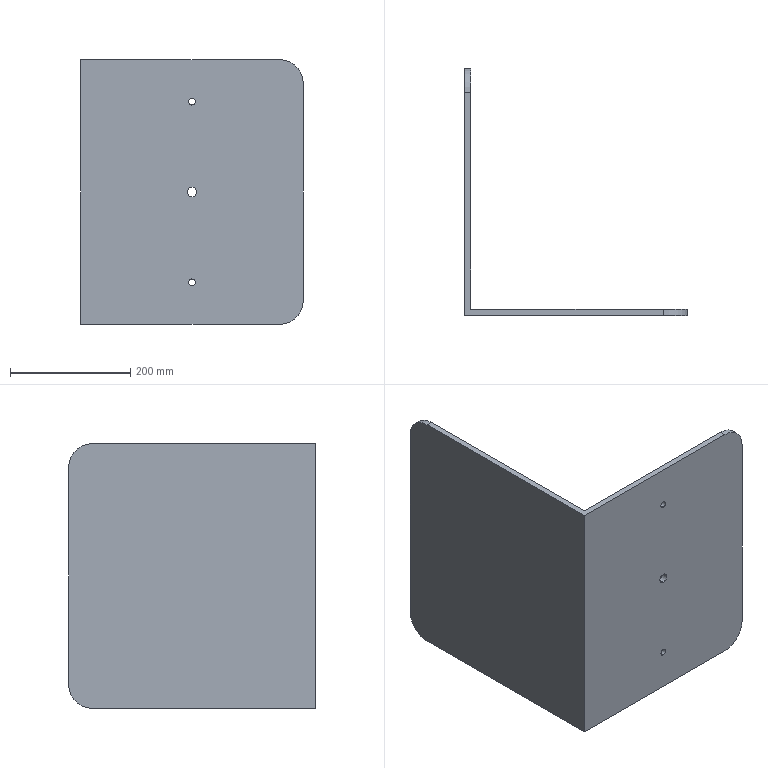Part | SolidWorks | features ICE 2, Extrusion 1, Fillet 1 | 1 solid | 18 faces | box 370 x 410 x 440 mm | volume 3370354 mm3 | cylinder 10 | plane 8 | commonest cylinder face diameters 11 x4 80 x4 16 x2
STEP:
#1=CARTESIAN_POINT('',(0.,-5.,155.5));
#2=VERTEX_POINT('',#1);
#3=CARTESIAN_POINT('',(0.,-5.,144.5));
#4=VERTEX_POINT('',#3);
#5=CARTESIAN_POINT('',(0.,-5.,150.));
#6=DIRECTION('',(0.,-1.,0.));
#7=DIRECTION('',(0.,0.,1.));
#8=AXIS2_PLACEMENT_3D('',#5,#6,#7);
#9=CIRCLE('',#8,5.5);
#10=EDGE_CURVE('',#2,#4,#9,.T.);
#11=ORIENTED_EDGE('',*,*,#10,.T.);
#12=CARTESIAN_POINT('',(0.,5.,144.5));
#13=VERTEX_POINT('',#12);
#14=CARTESIAN_POINT('',(0.,-5.001,144.5));
#15=DIRECTION('',(0.,1.,0.));
#16=VECTOR('',#15,1000.);
#17=LINE('',#14,#16);
#18=EDGE_CURVE('',#4,#13,#17,.T.);
#19=ORIENTED_EDGE('',*,*,#18,.T.);
#20=CARTESIAN_POINT('',(0.,5.,155.5));
#21=VERTEX_POINT('',#20);
#22=CARTESIAN_POINT('',(0.,5.,150.));
#23=DIRECTION('',(0.,1.,0.));
#24=DIRECTION('',(0.,0.,-1.));
#25=AXIS2_PLACEMENT_3D('',#22,#23,#24);
#26=CIRCLE('',#25,5.5);
#27=EDGE_CURVE('',#13,#21,#26,.T.);
#28=ORIENTED_EDGE('',*,*,#27,.T.);
#29=CARTESIAN_POINT('',(0.,-5.001,155.5));
#30=DIRECTION('',(0.,1.,0.));
#31=VECTOR('',#30,1000.);
#32=LINE('',#29,#31);
#33=EDGE_CURVE('',#2,#21,#32,.T.);
#34=ORIENTED_EDGE('',*,*,#33,.F.);
#35=EDGE_LOOP('',(#11,#19,#28,#34));
#36=FACE_OUTER_BOUND('',#35,.T.);
#37=CARTESIAN_POINT('',(0.,-5.001,150.));
#38=DIRECTION('',(0.,1.,0.));
#39=DIRECTION('',(0.,0.,1.));
#40=AXIS2_PLACEMENT_3D('',#37,#38,#39);
#41=CYLINDRICAL_SURFACE('',#40,5.5);
#42=ADVANCED_FACE('',(#36),#41,.F.);
#43=CARTESIAN_POINT('',(0.,-5.,-144.5));
#44=VERTEX_POINT('',#43);
#45=CARTESIAN_POINT('',(0.,-5.,-155.5));
#46=VERTEX_POINT('',#45);
#47=CARTESIAN_POINT('',(0.,-5.,-150.));
#48=DIRECTION('',(0.,-1.,0.));
#49=DIRECTION('',(0.,0.,1.));
#50=AXIS2_PLACEMENT_3D('',#47,#48,#49);
#51=CIRCLE('',#50,5.5);
#52=EDGE_CURVE('',#44,#46,#51,.T.);
#53=ORIENTED_EDGE('',*,*,#52,.T.);
#54=CARTESIAN_POINT('',(0.,5.,-155.5));
#55=VERTEX_POINT('',#54);
#56=CARTESIAN_POINT('',(0.,-5.001,-155.5));
#57=DIRECTION('',(0.,1.,0.));
#58=VECTOR('',#57,1000.);
#59=LINE('',#56,#58);
#60=EDGE_CURVE('',#46,#55,#59,.T.);
#61=ORIENTED_EDGE('',*,*,#60,.T.);
#62=CARTESIAN_POINT('',(0.,5.,-144.5));
#63=VERTEX_POINT('',#62);
#64=CARTESIAN_POINT('',(0.,5.,-150.));
#65=DIRECTION('',(0.,1.,0.));
#66=DIRECTION('',(0.,0.,1.));
#67=AXIS2_PLACEMENT_3D('',#64,#65,#66);
#68=CIRCLE('',#67,5.5);
#69=EDGE_CURVE('',#55,#63,#68,.T.);
#70=ORIENTED_EDGE('',*,*,#69,.T.);
#71=CARTESIAN_POINT('',(0.,-5.001,-144.5));
#72=DIRECTION('',(0.,1.,0.));
#73=VECTOR('',#72,1000.);
#74=LINE('',#71,#73);
#75=EDGE_CURVE('',#44,#63,#74,.T.);
#76=ORIENTED_EDGE('',*,*,#75,.F.);
#77=EDGE_LOOP('',(#53,#61,#70,#76));
#78=FACE_OUTER_BOUND('',#77,.T.);
#79=CARTESIAN_POINT('',(0.,-5.001,-150.));
#80=DIRECTION('',(0.,1.,0.));
#81=DIRECTION('',(0.,0.,1.));
#82=AXIS2_PLACEMENT_3D('',#79,#80,#81);
#83=CYLINDRICAL_SURFACE('',#82,5.5);
#84=ADVANCED_FACE('',(#78),#83,.F.);
#85=CARTESIAN_POINT('',(0.,-5.,8.));
#86=VERTEX_POINT('',#85);
#87=CARTESIAN_POINT('',(0.,-5.,-8.));
#88=VERTEX_POINT('',#87);
#89=CARTESIAN_POINT('',(0.,-5.,0.));
#90=DIRECTION('',(0.,-1.,0.));
#91=DIRECTION('',(0.,0.,1.));
#92=AXIS2_PLACEMENT_3D('',#89,#90,#91);
#93=CIRCLE('',#92,8.);
#94=EDGE_CURVE('',#86,#88,#93,.T.);
#95=ORIENTED_EDGE('',*,*,#94,.T.);
#96=CARTESIAN_POINT('',(0.,5.,-8.));
#97=VERTEX_POINT('',#96);
#98=CARTESIAN_POINT('',(0.,-5.001,-8.));
#99=DIRECTION('',(0.,1.,0.));
#100=VECTOR('',#99,1000.);
#101=LINE('',#98,#100);
#102=EDGE_CURVE('',#88,#97,#101,.T.);
#103=ORIENTED_EDGE('',*,*,#102,.T.);
#104=CARTESIAN_POINT('',(0.,5.,8.));
#105=VERTEX_POINT('',#104);
#106=CARTESIAN_POINT('',(0.,5.,0.));
#107=DIRECTION('',(0.,1.,0.));
#108=DIRECTION('',(0.,0.,1.));
#109=AXIS2_PLACEMENT_3D('',#106,#107,#108);
#110=CIRCLE('',#109,8.);
#111=EDGE_CURVE('',#97,#105,#110,.T.);
#112=ORIENTED_EDGE('',*,*,#111,.T.);
#113=CARTESIAN_POINT('',(0.,-5.001,8.));
#114=DIRECTION('',(0.,1.,0.));
#115=VECTOR('',#114,1000.);
#116=LINE('',#113,#115);
#117=EDGE_CURVE('',#86,#105,#116,.T.);
#118=ORIENTED_EDGE('',*,*,#117,.F.);
#119=EDGE_LOOP('',(#95,#103,#112,#118));
#120=FACE_OUTER_BOUND('',#119,.T.);
#121=CARTESIAN_POINT('',(0.,-5.001,0.));
#122=DIRECTION('',(0.,1.,0.));
#123=DIRECTION('',(0.,0.,1.));
#124=AXIS2_PLACEMENT_3D('',#121,#122,#123);
#125=CYLINDRICAL_SURFACE('',#124,8.);
#126=ADVANCED_FACE('',(#120),#125,.F.);
#127=CARTESIAN_POINT('',(185.,-5.,180.));
#128=VERTEX_POINT('',#127);
#129=CARTESIAN_POINT('',(185.,-5.,-180.));
#130=VERTEX_POINT('',#129);
#131=CARTESIAN_POINT('',(185.,-5.,-220.));
#132=DIRECTION('',(0.,0.,-1.));
#133=VECTOR('',#132,1000.);
#134=LINE('',#131,#133);
#135=EDGE_CURVE('',#128,#130,#134,.T.);
#136=ORIENTED_EDGE('',*,*,#135,.T.);
#137=CARTESIAN_POINT('',(185.,5.,-180.));
#138=VERTEX_POINT('',#137);
#139=CARTESIAN_POINT('',(185.,5.,-180.));
#140=DIRECTION('',(0.,1.,0.));
#141=VECTOR('',#140,1000.);
#142=LINE('',#139,#141);
#143=EDGE_CURVE('',#130,#138,#142,.T.);
#144=ORIENTED_EDGE('',*,*,#143,.T.);
#145=CARTESIAN_POINT('',(185.,5.,180.));
#146=VERTEX_POINT('',#145);
#147=CARTESIAN_POINT('',(185.,5.,-220.));
#148=DIRECTION('',(0.,0.,-1.));
#149=VECTOR('',#148,1000.);
#150=LINE('',#147,#149);
#151=EDGE_CURVE('',#146,#138,#150,.T.);
#152=ORIENTED_EDGE('',*,*,#151,.F.);
#153=CARTESIAN_POINT('',(185.,5.,180.));
#154=DIRECTION('',(0.,-1.,0.));
#155=VECTOR('',#154,1000.);
#156=LINE('',#153,#155);
#157=EDGE_CURVE('',#146,#128,#156,.T.);
#158=ORIENTED_EDGE('',*,*,#157,.T.);
#159=EDGE_LOOP('',(#136,#144,#152,#158));
#160=FACE_OUTER_BOUND('',#159,.T.);
#161=CARTESIAN_POINT('',(185.,5.,-220.));
#162=DIRECTION('',(-1.,0.,0.));
#163=DIRECTION('',(0.,0.,1.));
#164=AXIS2_PLACEMENT_3D('',#161,#162,#163);
#165=PLANE('',#164);
#166=ADVANCED_FACE('',(#160),#165,.F.);
#167=CARTESIAN_POINT('',(-185.,365.,-220.));
#168=VERTEX_POINT('',#167);
#169=CARTESIAN_POINT('',(-185.,-5.,-220.));
#170=VERTEX_POINT('',#169);
#171=CARTESIAN_POINT('',(-185.,5.,-220.));
#172=DIRECTION('',(0.,-1.,0.));
#173=VECTOR('',#172,1000.);
#174=LINE('',#171,#173);
#175=EDGE_CURVE('',#168,#170,#174,.T.);
#176=ORIENTED_EDGE('',*,*,#175,.F.);
#177=CARTESIAN_POINT('',(-175.,365.,-220.));
#178=VERTEX_POINT('',#177);
#179=CARTESIAN_POINT('',(-175.,365.,-220.));
#180=DIRECTION('',(1.,0.,0.));
#181=VECTOR('',#180,1000.);
#182=LINE('',#179,#181);
#183=EDGE_CURVE('',#168,#178,#182,.T.);
#184=ORIENTED_EDGE('',*,*,#183,.T.);
#185=CARTESIAN_POINT('',(-175.,5.,-220.));
#186=VERTEX_POINT('',#185);
#187=CARTESIAN_POINT('',(-175.,405.,-220.));
#188=DIRECTION('',(0.,-1.,0.));
#189=VECTOR('',#188,1000.);
#190=LINE('',#187,#189);
#191=EDGE_CURVE('',#178,#186,#190,.T.);
#192=ORIENTED_EDGE('',*,*,#191,.T.);
#193=CARTESIAN_POINT('',(145.,5.,-220.));
#194=VERTEX_POINT('',#193);
#195=CARTESIAN_POINT('',(-185.,5.,-220.));
#196=DIRECTION('',(-1.,0.,0.));
#197=VECTOR('',#196,1000.);
#198=LINE('',#195,#197);
#199=EDGE_CURVE('',#194,#186,#198,.T.);
#200=ORIENTED_EDGE('',*,*,#199,.F.);
#201=CARTESIAN_POINT('',(145.,-5.,-220.));
#202=VERTEX_POINT('',#201);
#203=CARTESIAN_POINT('',(145.,5.,-220.));
#204=DIRECTION('',(0.,-1.,0.));
#205=VECTOR('',#204,1000.);
#206=LINE('',#203,#205);
#207=EDGE_CURVE('',#194,#202,#206,.T.);
#208=ORIENTED_EDGE('',*,*,#207,.T.);
#209=CARTESIAN_POINT('',(-185.,-5.,-220.));
#210=DIRECTION('',(-1.,0.,0.));
#211=VECTOR('',#210,1000.);
#212=LINE('',#209,#211);
#213=EDGE_CURVE('',#202,#170,#212,.T.);
#214=ORIENTED_EDGE('',*,*,#213,.T.);
#215=EDGE_LOOP('',(#176,#184,#192,#200,#208,#214));
#216=FACE_OUTER_BOUND('',#215,.T.);
#217=CARTESIAN_POINT('',(-185.,5.,-220.));
#218=DIRECTION('',(0.,0.,1.));
#219=DIRECTION('',(1.,0.,0.));
#220=AXIS2_PLACEMENT_3D('',#217,#218,#219);
#221=PLANE('',#220);
#222=ADVANCED_FACE('',(#216),#221,.F.);
#223=CARTESIAN_POINT('',(-185.,405.,-180.));
#224=VERTEX_POINT('',#223);
#225=CARTESIAN_POINT('',(-185.,405.,180.));
#226=VERTEX_POINT('',#225);
#227=CARTESIAN_POINT('',(-185.,405.,-220.));
#228=DIRECTION('',(0.,0.,1.));
#229=VECTOR('',#228,1000.);
#230=LINE('',#227,#229);
#231=EDGE_CURVE('',#224,#226,#230,.T.);
#232=ORIENTED_EDGE('',*,*,#231,.F.);
#233=CARTESIAN_POINT('',(-185.,365.,-180.));
#234=DIRECTION('',(-1.,0.,0.));
#235=DIRECTION('',(0.,0.,-1.));
#236=AXIS2_PLACEMENT_3D('',#233,#234,#235);
#237=CIRCLE('',#236,40.);
#238=EDGE_CURVE('',#224,#168,#237,.T.);
#239=ORIENTED_EDGE('',*,*,#238,.T.);
#240=ORIENTED_EDGE('',*,*,#175,.T.);
#241=CARTESIAN_POINT('',(-185.,-5.,220.));
#242=VERTEX_POINT('',#241);
#243=CARTESIAN_POINT('',(-185.,-5.,-220.));
#244=DIRECTION('',(0.,0.,1.));
#245=VECTOR('',#244,1000.);
#246=LINE('',#243,#245);
#247=EDGE_CURVE('',#170,#242,#246,.T.);
#248=ORIENTED_EDGE('',*,*,#247,.T.);
#249=CARTESIAN_POINT('',(-185.,365.,220.));
#250=VERTEX_POINT('',#249);
#251=CARTESIAN_POINT('',(-185.,5.,220.));
#252=DIRECTION('',(0.,-1.,0.));
#253=VECTOR('',#252,1000.);
#254=LINE('',#251,#253);
#255=EDGE_CURVE('',#250,#242,#254,.T.);
#256=ORIENTED_EDGE('',*,*,#255,.F.);
#257=CARTESIAN_POINT('',(-185.,365.,180.));
#258=DIRECTION('',(-1.,0.,0.));
#259=DIRECTION('',(0.,0.,-1.));
#260=AXIS2_PLACEMENT_3D('',#257,#258,#259);
#261=CIRCLE('',#260,40.);
#262=EDGE_CURVE('',#250,#226,#261,.T.);
#263=ORIENTED_EDGE('',*,*,#262,.T.);
#264=EDGE_LOOP('',(#232,#239,#240,#248,#256,#263));
#265=FACE_OUTER_BOUND('',#264,.T.);
#266=CARTESIAN_POINT('',(-185.,5.,-220.));
#267=DIRECTION('',(1.,0.,0.));
#268=DIRECTION('',(0.,0.,-1.));
#269=AXIS2_PLACEMENT_3D('',#266,#267,#268);
#270=PLANE('',#269);
#271=ADVANCED_FACE('',(#265),#270,.F.);
#272=CARTESIAN_POINT('',(-175.,365.,220.));
#273=VERTEX_POINT('',#272);
#274=CARTESIAN_POINT('',(-175.,5.,220.));
#275=VERTEX_POINT('',#274);
#276=CARTESIAN_POINT('',(-175.,405.,220.));
#277=DIRECTION('',(0.,-1.,0.));
#278=VECTOR('',#277,1000.);
#279=LINE('',#276,#278);
#280=EDGE_CURVE('',#273,#275,#279,.T.);
#281=ORIENTED_EDGE('',*,*,#280,.F.);
#282=CARTESIAN_POINT('',(-185.,365.,220.));
#283=DIRECTION('',(-1.,0.,0.));
#284=VECTOR('',#283,1000.);
#285=LINE('',#282,#284);
#286=EDGE_CURVE('',#273,#250,#285,.T.);
#287=ORIENTED_EDGE('',*,*,#286,.T.);
#288=ORIENTED_EDGE('',*,*,#255,.T.);
#289=CARTESIAN_POINT('',(145.,-5.,220.));
#290=VERTEX_POINT('',#289);
#291=CARTESIAN_POINT('',(-185.,-5.,220.));
#292=DIRECTION('',(1.,0.,0.));
#293=VECTOR('',#292,1000.);
#294=LINE('',#291,#293);
#295=EDGE_CURVE('',#242,#290,#294,.T.);
#296=ORIENTED_EDGE('',*,*,#295,.T.);
#297=CARTESIAN_POINT('',(145.,5.,220.));
#298=VERTEX_POINT('',#297);
#299=CARTESIAN_POINT('',(145.,5.,220.));
#300=DIRECTION('',(0.,1.,0.));
#301=VECTOR('',#300,1000.);
#302=LINE('',#299,#301);
#303=EDGE_CURVE('',#290,#298,#302,.T.);
#304=ORIENTED_EDGE('',*,*,#303,.T.);
#305=CARTESIAN_POINT('',(-185.,5.,220.));
#306=DIRECTION('',(1.,0.,0.));
#307=VECTOR('',#306,1000.);
#308=LINE('',#305,#307);
#309=EDGE_CURVE('',#275,#298,#308,.T.);
#310=ORIENTED_EDGE('',*,*,#309,.F.);
#311=EDGE_LOOP('',(#281,#287,#288,#296,#304,#310));
#312=FACE_OUTER_BOUND('',#311,.T.);
#313=CARTESIAN_POINT('',(-185.,5.,220.));
#314=DIRECTION('',(0.,0.,-1.));
#315=DIRECTION('',(-1.,0.,0.));
#316=AXIS2_PLACEMENT_3D('',#313,#314,#315);
#317=PLANE('',#316);
#318=ADVANCED_FACE('',(#312),#317,.F.);
#319=ORIENTED_EDGE('',*,*,#151,.T.);
#320=CARTESIAN_POINT('',(145.,5.,-180.));
#321=DIRECTION('',(0.,1.,0.));
#322=DIRECTION('',(0.,0.,1.));
#323=AXIS2_PLACEMENT_3D('',#320,#321,#322);
#324=CIRCLE('',#323,40.);
#325=EDGE_CURVE('',#138,#194,#324,.T.);
#326=ORIENTED_EDGE('',*,*,#325,.T.);
#327=ORIENTED_EDGE('',*,*,#199,.T.);
#328=CARTESIAN_POINT('',(-175.,5.,-220.));
#329=DIRECTION('',(0.,0.,-1.));
#330=VECTOR('',#329,1000.);
#331=LINE('',#328,#330);
#332=EDGE_CURVE('',#275,#186,#331,.T.);
#333=ORIENTED_EDGE('',*,*,#332,.F.);
#334=ORIENTED_EDGE('',*,*,#309,.T.);
#335=CARTESIAN_POINT('',(145.,5.,180.));
#336=DIRECTION('',(0.,1.,0.));
#337=DIRECTION('',(0.,0.,1.));
#338=AXIS2_PLACEMENT_3D('',#335,#336,#337);
#339=CIRCLE('',#338,40.);
#340=EDGE_CURVE('',#298,#146,#339,.T.);
#341=ORIENTED_EDGE('',*,*,#340,.T.);
#342=EDGE_LOOP('',(#319,#326,#327,#333,#334,#341));
#343=FACE_OUTER_BOUND('',#342,.T.);
#344=CARTESIAN_POINT('',(0.,5.,150.));
#345=DIRECTION('',(0.,1.,0.));
#346=DIRECTION('',(0.,0.,-1.));
#347=AXIS2_PLACEMENT_3D('',#344,#345,#346);
#348=CIRCLE('',#347,5.5);
#349=EDGE_CURVE('',#21,#13,#348,.T.);
#350=ORIENTED_EDGE('',*,*,#349,.F.);
#351=ORIENTED_EDGE('',*,*,#27,.F.);
#352=EDGE_LOOP('',(#350,#351));
#353=FACE_BOUND('',#352,.T.);
#354=CARTESIAN_POINT('',(0.,5.,-150.));
#355=DIRECTION('',(0.,1.,0.));
#356=DIRECTION('',(0.,0.,1.));
#357=AXIS2_PLACEMENT_3D('',#354,#355,#356);
#358=CIRCLE('',#357,5.5);
#359=EDGE_CURVE('',#63,#55,#358,.T.);
#360=ORIENTED_EDGE('',*,*,#359,.F.);
#361=ORIENTED_EDGE('',*,*,#69,.F.);
#362=EDGE_LOOP('',(#360,#361));
#363=FACE_BOUND('',#362,.T.);
#364=CARTESIAN_POINT('',(0.,5.,0.));
#365=DIRECTION('',(0.,1.,0.));
#366=DIRECTION('',(0.,0.,1.));
#367=AXIS2_PLACEMENT_3D('',#364,#365,#366);
#368=CIRCLE('',#367,8.);
#369=EDGE_CURVE('',#105,#97,#368,.T.);
#370=ORIENTED_EDGE('',*,*,#369,.F.);
#371=ORIENTED_EDGE('',*,*,#111,.F.);
#372=EDGE_LOOP('',(#370,#371));
#373=FACE_BOUND('',#372,.T.);
#374=CARTESIAN_POINT('',(0.,5.,0.));
#375=DIRECTION('',(0.,1.,0.));
#376=DIRECTION('',(0.,0.,1.));
#377=AXIS2_PLACEMENT_3D('',#374,#375,#376);
#378=PLANE('',#377);
#379=ADVANCED_FACE('',(#343,#353,#363,#373),#378,.T.);
#380=ORIENTED_EDGE('',*,*,#10,.F.);
#381=CARTESIAN_POINT('',(0.,-5.,150.));
#382=DIRECTION('',(0.,-1.,0.));
#383=DIRECTION('',(0.,0.,1.));
#384=AXIS2_PLACEMENT_3D('',#381,#382,#383);
#385=CIRCLE('',#384,5.5);
#386=EDGE_CURVE('',#4,#2,#385,.T.);
#387=ORIENTED_EDGE('',*,*,#386,.F.);
#388=EDGE_LOOP('',(#380,#387));
#389=FACE_BOUND('',#388,.T.);
#390=ORIENTED_EDGE('',*,*,#52,.F.);
#391=CARTESIAN_POINT('',(0.,-5.,-150.));
#392=DIRECTION('',(0.,-1.,0.));
#393=DIRECTION('',(0.,0.,1.));
#394=AXIS2_PLACEMENT_3D('',#391,#392,#393);
#395=CIRCLE('',#394,5.5);
#396=EDGE_CURVE('',#46,#44,#395,.T.);
#397=ORIENTED_EDGE('',*,*,#396,.F.);
#398=EDGE_LOOP('',(#390,#397));
#399=FACE_BOUND('',#398,.T.);
#400=ORIENTED_EDGE('',*,*,#94,.F.);
#401=CARTESIAN_POINT('',(0.,-5.,0.));
#402=DIRECTION('',(0.,-1.,0.));
#403=DIRECTION('',(0.,0.,1.));
#404=AXIS2_PLACEMENT_3D('',#401,#402,#403);
#405=CIRCLE('',#404,8.);
#406=EDGE_CURVE('',#88,#86,#405,.T.);
#407=ORIENTED_EDGE('',*,*,#406,.F.);
#408=EDGE_LOOP('',(#400,#407));
#409=FACE_BOUND('',#408,.T.);
#410=ORIENTED_EDGE('',*,*,#213,.F.);
#411=CARTESIAN_POINT('',(145.,-5.,-180.));
#412=DIRECTION('',(0.,-1.,0.));
#413=DIRECTION('',(0.,0.,1.));
#414=AXIS2_PLACEMENT_3D('',#411,#412,#413);
#415=CIRCLE('',#414,40.);
#416=EDGE_CURVE('',#202,#130,#415,.T.);
#417=ORIENTED_EDGE('',*,*,#416,.T.);
#418=ORIENTED_EDGE('',*,*,#135,.F.);
#419=CARTESIAN_POINT('',(145.,-5.,180.));
#420=DIRECTION('',(0.,-1.,0.));
#421=DIRECTION('',(0.,0.,1.));
#422=AXIS2_PLACEMENT_3D('',#419,#420,#421);
#423=CIRCLE('',#422,40.);
#424=EDGE_CURVE('',#128,#290,#423,.T.);
#425=ORIENTED_EDGE('',*,*,#424,.T.);
#426=ORIENTED_EDGE('',*,*,#295,.F.);
#427=ORIENTED_EDGE('',*,*,#247,.F.);
#428=EDGE_LOOP('',(#410,#417,#418,#425,#426,#427));
#429=FACE_OUTER_BOUND('',#428,.T.);
#430=CARTESIAN_POINT('',(0.,-5.,0.));
#431=DIRECTION('',(0.,1.,0.));
#432=DIRECTION('',(0.,0.,1.));
#433=AXIS2_PLACEMENT_3D('',#430,#431,#432);
#434=PLANE('',#433);
#435=ADVANCED_FACE('',(#389,#399,#409,#429),#434,.F.);
#436=ORIENTED_EDGE('',*,*,#102,.F.);
#437=ORIENTED_EDGE('',*,*,#406,.T.);
#438=ORIENTED_EDGE('',*,*,#117,.T.);
#439=ORIENTED_EDGE('',*,*,#369,.T.);
#440=EDGE_LOOP('',(#436,#437,#438,#439));
#441=FACE_OUTER_BOUND('',#440,.T.);
#442=CARTESIAN_POINT('',(0.,-5.001,0.));
#443=DIRECTION('',(0.,1.,0.));
#444=DIRECTION('',(0.,0.,1.));
#445=AXIS2_PLACEMENT_3D('',#442,#443,#444);
#446=CYLINDRICAL_SURFACE('',#445,8.);
#447=ADVANCED_FACE('',(#441),#446,.F.);
#448=ORIENTED_EDGE('',*,*,#60,.F.);
#449=ORIENTED_EDGE('',*,*,#396,.T.);
#450=ORIENTED_EDGE('',*,*,#75,.T.);
#451=ORIENTED_EDGE('',*,*,#359,.T.);
#452=EDGE_LOOP('',(#448,#449,#450,#451));
#453=FACE_OUTER_BOUND('',#452,.T.);
#454=CARTESIAN_POINT('',(0.,-5.001,-150.));
#455=DIRECTION('',(0.,1.,0.));
#456=DIRECTION('',(0.,0.,1.));
#457=AXIS2_PLACEMENT_3D('',#454,#455,#456);
#458=CYLINDRICAL_SURFACE('',#457,5.5);
#459=ADVANCED_FACE('',(#453),#458,.F.);
#460=ORIENTED_EDGE('',*,*,#18,.F.);
#461=ORIENTED_EDGE('',*,*,#386,.T.);
#462=ORIENTED_EDGE('',*,*,#33,.T.);
#463=ORIENTED_EDGE('',*,*,#349,.T.);
#464=EDGE_LOOP('',(#460,#461,#462,#463));
#465=FACE_OUTER_BOUND('',#464,.T.);
#466=CARTESIAN_POINT('',(0.,-5.001,150.));
#467=DIRECTION('',(0.,1.,0.));
#468=DIRECTION('',(0.,0.,1.));
#469=AXIS2_PLACEMENT_3D('',#466,#467,#468);
#470=CYLINDRICAL_SURFACE('',#469,5.5);
#471=ADVANCED_FACE('',(#465),#470,.F.);
#472=ORIENTED_EDGE('',*,*,#191,.F.);
#473=CARTESIAN_POINT('',(-175.,405.,-180.));
#474=VERTEX_POINT('',#473);
#475=CARTESIAN_POINT('',(-175.,365.,-180.));
#476=DIRECTION('',(1.,0.,0.));
#477=DIRECTION('',(0.,0.,1.));
#478=AXIS2_PLACEMENT_3D('',#475,#476,#477);
#479=CIRCLE('',#478,40.);
#480=EDGE_CURVE('',#178,#474,#479,.T.);
#481=ORIENTED_EDGE('',*,*,#480,.T.);
#482=CARTESIAN_POINT('',(-175.,405.,180.));
#483=VERTEX_POINT('',#482);
#484=CARTESIAN_POINT('',(-175.,405.,-220.));
#485=DIRECTION('',(0.,0.,-1.));
#486=VECTOR('',#485,1000.);
#487=LINE('',#484,#486);
#488=EDGE_CURVE('',#483,#474,#487,.T.);
#489=ORIENTED_EDGE('',*,*,#488,.F.);
#490=CARTESIAN_POINT('',(-175.,365.,180.));
#491=DIRECTION('',(1.,0.,0.));
#492=DIRECTION('',(0.,0.,1.));
#493=AXIS2_PLACEMENT_3D('',#490,#491,#492);
#494=CIRCLE('',#493,40.);
#495=EDGE_CURVE('',#483,#273,#494,.T.);
#496=ORIENTED_EDGE('',*,*,#495,.T.);
#497=ORIENTED_EDGE('',*,*,#280,.T.);
#498=ORIENTED_EDGE('',*,*,#332,.T.);
#499=EDGE_LOOP('',(#472,#481,#489,#496,#497,#498));
#500=FACE_OUTER_BOUND('',#499,.T.);
#501=CARTESIAN_POINT('',(-175.,405.,-220.));
#502=DIRECTION('',(-1.,0.,0.));
#503=DIRECTION('',(0.,0.,1.));
#504=AXIS2_PLACEMENT_3D('',#501,#502,#503);
#505=PLANE('',#504);
#506=ADVANCED_FACE('',(#500),#505,.F.);
#507=ORIENTED_EDGE('',*,*,#488,.T.);
#508=CARTESIAN_POINT('',(-185.,405.,-180.));
#509=DIRECTION('',(-1.,0.,0.));
#510=VECTOR('',#509,1000.);
#511=LINE('',#508,#510);
#512=EDGE_CURVE('',#474,#224,#511,.T.);
#513=ORIENTED_EDGE('',*,*,#512,.T.);
#514=ORIENTED_EDGE('',*,*,#231,.T.);
#515=CARTESIAN_POINT('',(-175.,405.,180.));
#516=DIRECTION('',(1.,0.,0.));
#517=VECTOR('',#516,1000.);
#518=LINE('',#515,#517);
#519=EDGE_CURVE('',#226,#483,#518,.T.);
#520=ORIENTED_EDGE('',*,*,#519,.T.);
#521=EDGE_LOOP('',(#507,#513,#514,#520));
#522=FACE_OUTER_BOUND('',#521,.T.);
#523=CARTESIAN_POINT('',(0.,405.,0.));
#524=DIRECTION('',(0.,1.,0.));
#525=DIRECTION('',(0.,0.,1.));
#526=AXIS2_PLACEMENT_3D('',#523,#524,#525);
#527=PLANE('',#526);
#528=ADVANCED_FACE('',(#522),#527,.T.);
#529=ORIENTED_EDGE('',*,*,#480,.F.);
#530=ORIENTED_EDGE('',*,*,#183,.F.);
#531=ORIENTED_EDGE('',*,*,#238,.F.);
#532=ORIENTED_EDGE('',*,*,#512,.F.);
#533=EDGE_LOOP('',(#529,#530,#531,#532));
#534=FACE_OUTER_BOUND('',#533,.T.);
#535=CARTESIAN_POINT('',(0.,365.,-180.));
#536=DIRECTION('',(1.,0.,0.));
#537=DIRECTION('',(0.,0.,-1.));
#538=AXIS2_PLACEMENT_3D('',#535,#536,#537);
#539=CYLINDRICAL_SURFACE('',#538,40.);
#540=ADVANCED_FACE('',(#534),#539,.T.);
#541=ORIENTED_EDGE('',*,*,#262,.F.);
#542=ORIENTED_EDGE('',*,*,#286,.F.);
#543=ORIENTED_EDGE('',*,*,#495,.F.);
#544=ORIENTED_EDGE('',*,*,#519,.F.);
#545=EDGE_LOOP('',(#541,#542,#543,#544));
#546=FACE_OUTER_BOUND('',#545,.T.);
#547=CARTESIAN_POINT('',(0.,365.,180.));
#548=DIRECTION('',(-1.,0.,0.));
#549=DIRECTION('',(0.,0.,1.));
#550=AXIS2_PLACEMENT_3D('',#547,#548,#549);
#551=CYLINDRICAL_SURFACE('',#550,40.);
#552=ADVANCED_FACE('',(#546),#551,.T.);
#553=ORIENTED_EDGE('',*,*,#325,.F.);
#554=ORIENTED_EDGE('',*,*,#143,.F.);
#555=ORIENTED_EDGE('',*,*,#416,.F.);
#556=ORIENTED_EDGE('',*,*,#207,.F.);
#557=EDGE_LOOP('',(#553,#554,#555,#556));
#558=FACE_OUTER_BOUND('',#557,.T.);
#559=CARTESIAN_POINT('',(145.,5.,-180.));
#560=DIRECTION('',(0.,-1.,0.));
#561=DIRECTION('',(0.,0.,-1.));
#562=AXIS2_PLACEMENT_3D('',#559,#560,#561);
#563=CYLINDRICAL_SURFACE('',#562,40.);
#564=ADVANCED_FACE('',(#558),#563,.T.);
#565=ORIENTED_EDGE('',*,*,#340,.F.);
#566=ORIENTED_EDGE('',*,*,#303,.F.);
#567=ORIENTED_EDGE('',*,*,#424,.F.);
#568=ORIENTED_EDGE('',*,*,#157,.F.);
#569=EDGE_LOOP('',(#565,#566,#567,#568));
#570=FACE_OUTER_BOUND('',#569,.T.);
#571=CARTESIAN_POINT('',(145.,5.,180.));
#572=DIRECTION('',(0.,-1.,0.));
#573=DIRECTION('',(0.,0.,-1.));
#574=AXIS2_PLACEMENT_3D('',#571,#572,#573);
#575=CYLINDRICAL_SURFACE('',#574,40.);
#576=ADVANCED_FACE('',(#570),#575,.T.);
#577=CLOSED_SHELL('',(#42,#84,#126,#166,#222,#271,#318,#379,#435,#447,#459,#471,#506,#528,#540,#552,#564,#576));
#578=MANIFOLD_SOLID_BREP('',#577);
#579=CARTESIAN_POINT('',(0.,0.,0.));
#580=DIRECTION('',(0.,0.,1.));
#581=DIRECTION('',(1.,0.,0.));
#582=AXIS2_PLACEMENT_3D('',#579,#580,#581);
#583=(LENGTH_UNIT()NAMED_UNIT(*)SI_UNIT(.MILLI.,.METRE.));
#584=UNCERTAINTY_MEASURE_WITH_UNIT(LENGTH_MEASURE(0.00001),#583,'','');
#585=(NAMED_UNIT(*)PLANE_ANGLE_UNIT()SI_UNIT($,.RADIAN.));
#586=(NAMED_UNIT(*)SI_UNIT($,.STERADIAN.)SOLID_ANGLE_UNIT());
#587=(GEOMETRIC_REPRESENTATION_CONTEXT(3)GLOBAL_UNCERTAINTY_ASSIGNED_CONTEXT((#584))GLOBAL_UNIT_ASSIGNED_CONTEXT((#583,#585,#586))REPRESENTATION_CONTEXT('',''));
#588=ADVANCED_BREP_SHAPE_REPRESENTATION('',(#578,#582),#587);